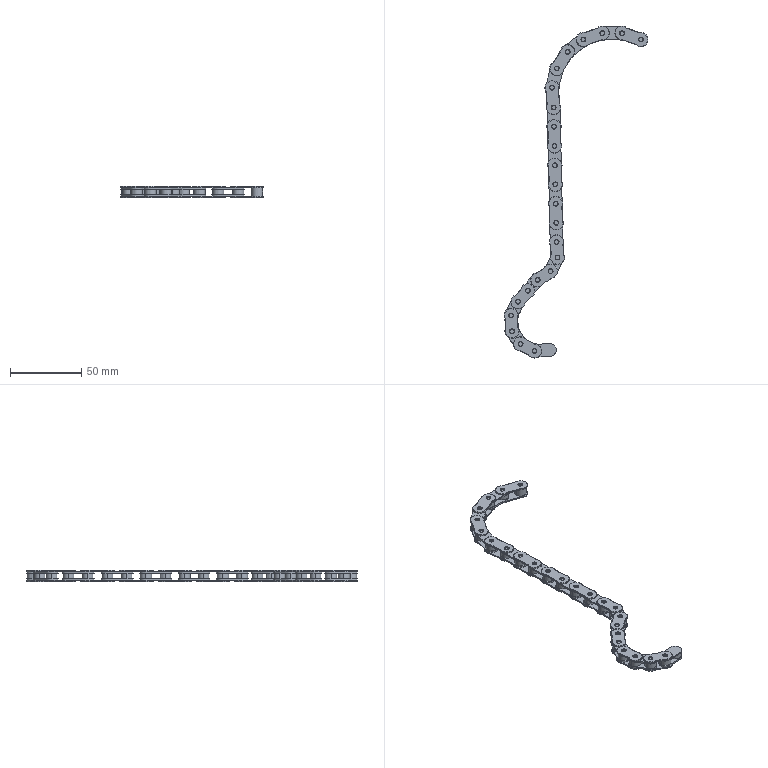Part | STEP file | Gear & derail Chain v2 | 1 solid | 818 faces | box 101.112 x 233.136 x 8 mm | volume 13651 mm3 | cylinder 374 | plane 240 | torus 204 | commonest cylinder face diameters 10 x108 3 x96 9 x72 8 x50 0.4 x48